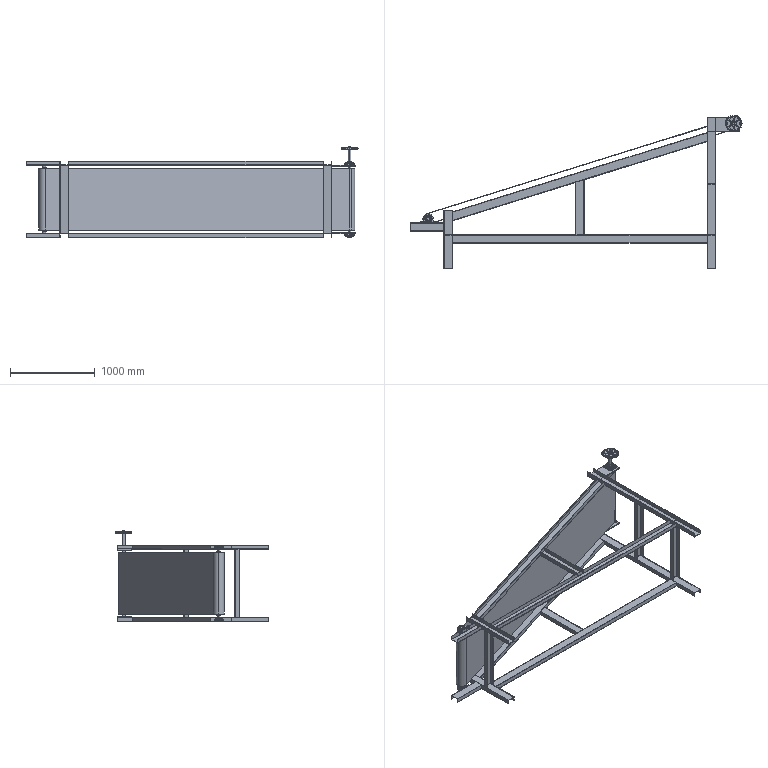Part | SolidWorks | features MirrorCompFeat 2, ReferencePattern 2 | 9 solids | 998 faces | box 3909 x 1808 x 1083 mm | volume 53217472 mm3 | plane 426 | cylinder 400 | torus 80 | cone 50 | sphere 36 | spline 6 | commonest cylinder face diameters 23.032 x49 41.467 x48 13 x32 16.059 x30 6 x28 26 x24